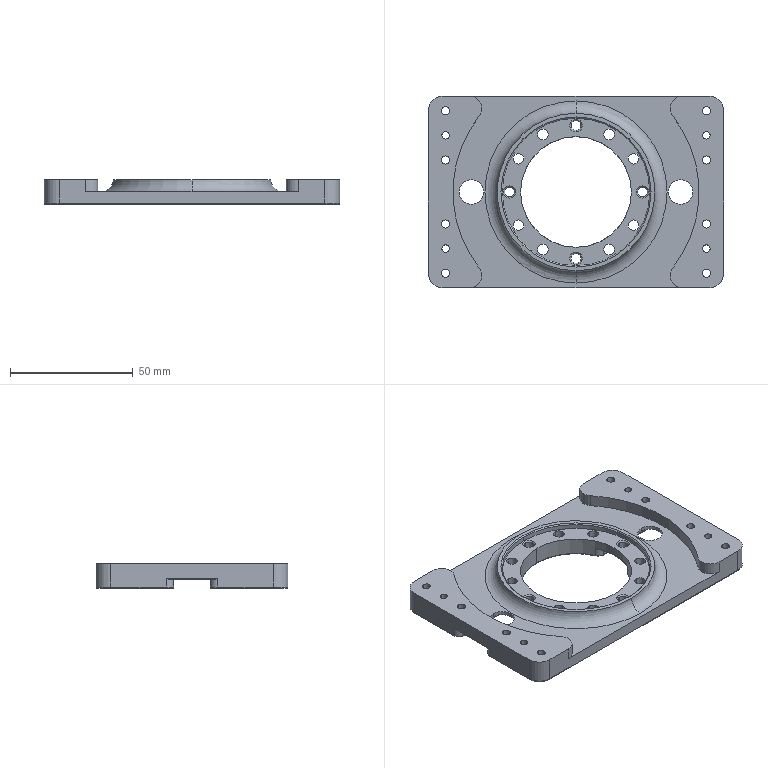NC program | NX | posted with a generic post | part box 120 x 78 x 10 mm
Lines 1 to 124 of 5508:
N10 G17 G21 G94 G90
(FLOOR_WALL , TOOL : D80)
N12 T19 M6
N14 G54
N16 G17 G0 G90 X-106.5 Y42.497 B0. C0. S6500 M3
N18 G43 Z30. H19
N20 Z3.
N22 G94 G1 Z0. F1500.
N24 X-103.5
N26 X103.5
N28 Y15.999
N30 X-103.5
N32 Y-10.5
N34 X103.5
N36 X106.5
N38 Z3.
N40 G0 Z30.
N42 M5
(DRILLING , TOOL : D6A45)
N44 T01 M6
N46 G54
N48 G17 G0 G90 X-53. Y-33. B0. C0. S5000 M3
N50 G43 Z30. H1
N52 G94 G81 G98 Z-1. F350. R3.
N54 Y-13.
N56 X-42.5 Y0.
N58 X-53. Y13.
N60 Y33.
N62 X-13.5 Y23.383
N64 X-23.383 Y13.5
N66 X-27. Y0.
N68 X-23.383 Y-13.5
N70 X-13.5 Y-23.383
N72 X13.5
N74 X23.383 Y-13.5
N76 X27. Y0.
N78 X23.383 Y13.5
N80 X13.5 Y23.383
N82 X53. Y33.
N84 Y13.
N86 X42.5 Y0.
N88 X53. Y-13.
N90 Y-33.
N92 G80
N94 G0 X53. Y-33. Z30.
(DRILLING_COPY_1 , TOOL : D6A45)
N96 Y23.
N98 G81 Z-2.5 F350. R3.
N100 Y-23.
N102 X0. Y-27.
N104 X-53. Y-23.
N106 Y23.
N108 X0. Y27.
N110 G80
N112 G0 X0. Y27. Z30.
N114 M5
(DRILLING_COPY , TOOL : 3.3ZT)
N116 T03 M6
N118 G54
N120 G17 G0 G90 X-53. Y-33. B0. C0. S2000 M3
N122 G43 Z30. H3
N124 G94 G83 G98 Z-11.991 F180. Q2. R3.
N126 Y-13.
N128 Y13.
N130 Y33.
N132 X53.
N134 Y13.
N136 Y-13.
N138 Y-33.
N140 G80
N142 G0 X53. Y-33. Z30.
(DRILLING_COPY_COPY_1 , TOOL : 3.3ZT)
N144 X27. Y0.
N146 G83 Z-11.991 F180. Q2. R3.
N148 X0. Y27.
N150 X-27. Y0.
N152 X0. Y-27.
N154 G80
N156 G0 X0. Y-27. Z30.
N158 M5
(DRILLING_COPY_COPY_1_COPY , TOOL : 2.5ZT)
N160 T02 M6
N162 G54
N164 G17 G0 G90 X-53. Y-23. B0. C0. S2000 M3
N166 G43 Z30. H2
N168 G94 G83 G98 Z-11.751 F120. Q2. R3.
N170 Y23.
N172 X53.
N174 Y-23.
N176 G80
N178 G0 X53. Y-23. Z30.
N180 M5
(DRILLING_COPY_COPY , TOOL : 4.3ZT)
N182 T16 M6
N184 G54
N186 G17 G0 G90 X23.383 Y13.5 B0. C0. S2000 M3
N188 G43 Z30. H16
N190 G94 G83 G98 Z-12.292 F180. Q2. R3.
N192 X13.5 Y23.383
N194 X-13.5
N196 X-23.383 Y13.5
N198 Y-13.5
N200 X-13.5 Y-23.383
N202 X13.5
N204 X23.383 Y-13.5
N206 G80
N208 G0 X23.383 Y-13.5 Z30.
N210 M5